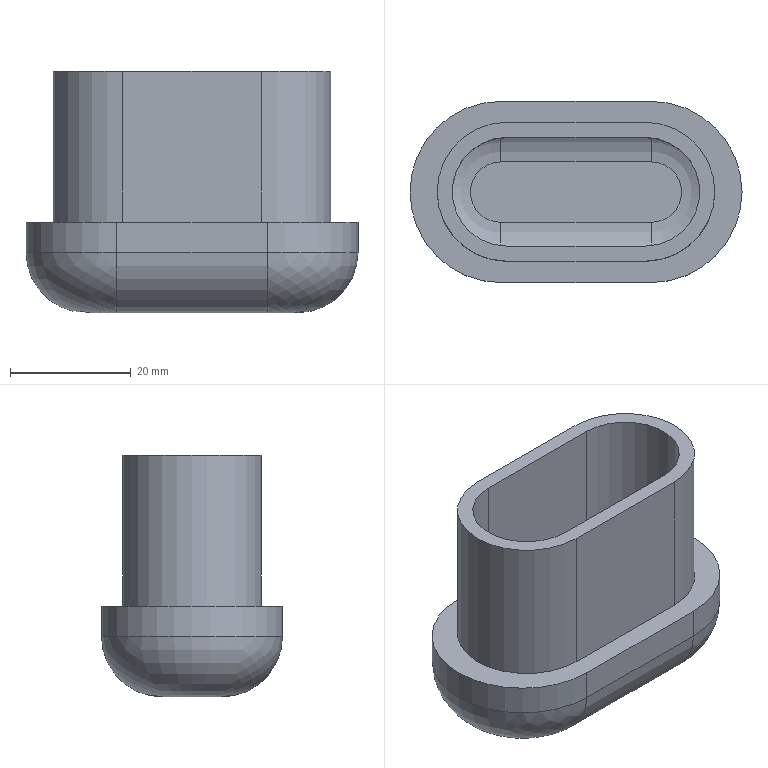Part | STEP file | 5091201W | 1 solid | 29 faces | box 55 x 30 x 40 mm | volume 14553 mm3 | plane 13 | cylinder 12 | other 4 | commonest cylinder face diameters 15 x2 18 x2 20 x2 23 x2 25 x2 30 x2